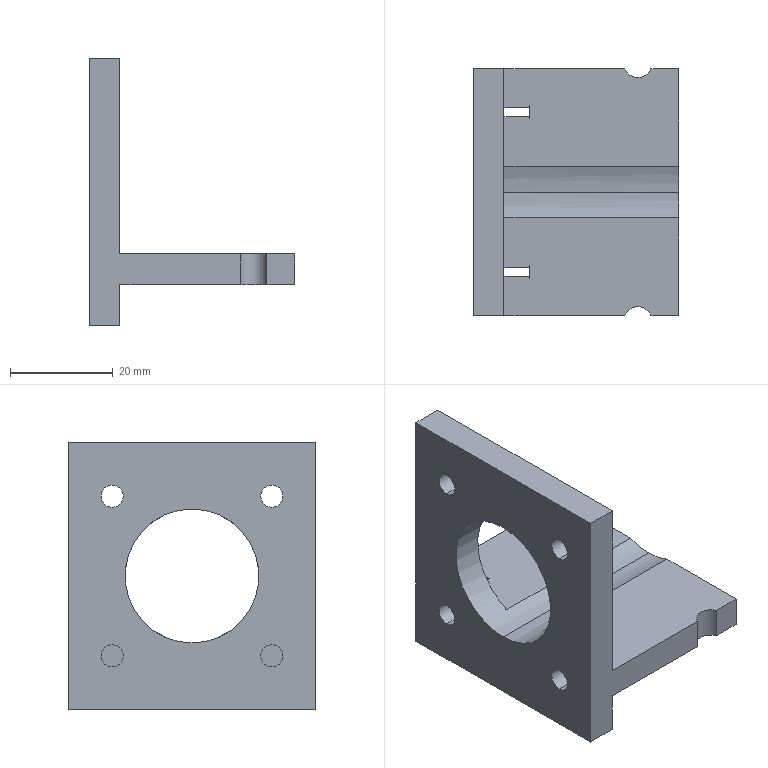Part | SolidWorks | features BaseBody 1 | 1 solid | 30 faces | box 40 x 48 x 52 mm | volume 20561 mm3 | cylinder 16 | plane 14 | commonest cylinder face diameters 4.3 x8 7.2 x4 5.5 x2 26 x2
STEP:
#1=CARTESIAN_POINT('',(0.,-15.5,31.35));
#2=VERTEX_POINT('',#1);
#3=CARTESIAN_POINT('',(0.,-15.5,35.65));
#4=VERTEX_POINT('',#3);
#5=CARTESIAN_POINT('',(0.,-15.5,33.5));
#6=DIRECTION('',(-1.,0.,0.));
#7=DIRECTION('',(0.,0.,-1.));
#8=AXIS2_PLACEMENT_3D('',#5,#6,#7);
#9=CIRCLE('',#8,2.15);
#10=EDGE_CURVE('',#2,#4,#9,.T.);
#11=ORIENTED_EDGE('',*,*,#10,.T.);
#12=CARTESIAN_POINT('',(6.,-15.5,35.65));
#13=VERTEX_POINT('',#12);
#14=CARTESIAN_POINT('',(-6.2,-15.5,35.65));
#15=DIRECTION('',(1.,0.,0.));
#16=VECTOR('',#15,1000.);
#17=LINE('',#14,#16);
#18=EDGE_CURVE('',#4,#13,#17,.T.);
#19=ORIENTED_EDGE('',*,*,#18,.T.);
#20=CARTESIAN_POINT('',(6.,-15.5,31.35));
#21=VERTEX_POINT('',#20);
#22=CARTESIAN_POINT('',(6.,-15.5,33.5));
#23=DIRECTION('',(-1.,0.,0.));
#24=DIRECTION('',(0.,0.,-1.));
#25=AXIS2_PLACEMENT_3D('',#22,#23,#24);
#26=CIRCLE('',#25,2.15);
#27=EDGE_CURVE('',#21,#13,#26,.T.);
#28=ORIENTED_EDGE('',*,*,#27,.F.);
#29=CARTESIAN_POINT('',(-6.2,-15.5,31.35));
#30=DIRECTION('',(1.,0.,0.));
#31=VECTOR('',#30,1000.);
#32=LINE('',#29,#31);
#33=EDGE_CURVE('',#2,#21,#32,.T.);
#34=ORIENTED_EDGE('',*,*,#33,.F.);
#35=EDGE_LOOP('',(#11,#19,#28,#34));
#36=FACE_OUTER_BOUND('',#35,.T.);
#37=CARTESIAN_POINT('',(-6.2,-15.5,33.5));
#38=DIRECTION('',(1.,0.,0.));
#39=DIRECTION('',(0.,0.,-1.));
#40=AXIS2_PLACEMENT_3D('',#37,#38,#39);
#41=CYLINDRICAL_SURFACE('',#40,2.15);
#42=ADVANCED_FACE('',(#36),#41,.F.);
#43=CARTESIAN_POINT('',(0.,0.,5.));
#44=VERTEX_POINT('',#43);
#45=CARTESIAN_POINT('',(0.,0.,31.));
#46=VERTEX_POINT('',#45);
#47=CARTESIAN_POINT('',(0.,0.,18.));
#48=DIRECTION('',(-1.,0.,0.));
#49=DIRECTION('',(0.,0.,-1.));
#50=AXIS2_PLACEMENT_3D('',#47,#48,#49);
#51=CIRCLE('',#50,13.);
#52=EDGE_CURVE('',#44,#46,#51,.T.);
#53=ORIENTED_EDGE('',*,*,#52,.T.);
#54=CARTESIAN_POINT('',(6.,0.,31.));
#55=VERTEX_POINT('',#54);
#56=CARTESIAN_POINT('',(-2.,0.,31.));
#57=DIRECTION('',(1.,0.,0.));
#58=VECTOR('',#57,1000.);
#59=LINE('',#56,#58);
#60=EDGE_CURVE('',#46,#55,#59,.T.);
#61=ORIENTED_EDGE('',*,*,#60,.T.);
#62=CARTESIAN_POINT('',(6.,-5.,6.));
#63=VERTEX_POINT('',#62);
#64=CARTESIAN_POINT('',(6.,0.,18.));
#65=DIRECTION('',(-1.,0.,0.));
#66=DIRECTION('',(0.,0.,-1.));
#67=AXIS2_PLACEMENT_3D('',#64,#65,#66);
#68=CIRCLE('',#67,13.);
#69=EDGE_CURVE('',#63,#55,#68,.T.);
#70=ORIENTED_EDGE('',*,*,#69,.F.);
#71=CARTESIAN_POINT('',(40.,-5.,6.));
#72=VERTEX_POINT('',#71);
#73=CARTESIAN_POINT('',(-2.,-5.,6.));
#74=DIRECTION('',(-1.,0.,0.));
#75=VECTOR('',#74,1000.);
#76=LINE('',#73,#75);
#77=EDGE_CURVE('',#72,#63,#76,.T.);
#78=ORIENTED_EDGE('',*,*,#77,.F.);
#79=CARTESIAN_POINT('',(40.,0.,5.));
#80=VERTEX_POINT('',#79);
#81=CARTESIAN_POINT('',(40.,0.,18.));
#82=DIRECTION('',(-1.,0.,0.));
#83=DIRECTION('',(0.,0.,-1.));
#84=AXIS2_PLACEMENT_3D('',#81,#82,#83);
#85=CIRCLE('',#84,13.);
#86=EDGE_CURVE('',#80,#72,#85,.T.);
#87=ORIENTED_EDGE('',*,*,#86,.F.);
#88=CARTESIAN_POINT('',(-2.,0.,5.));
#89=DIRECTION('',(1.,0.,0.));
#90=VECTOR('',#89,1000.);
#91=LINE('',#88,#90);
#92=EDGE_CURVE('',#44,#80,#91,.T.);
#93=ORIENTED_EDGE('',*,*,#92,.F.);
#94=EDGE_LOOP('',(#53,#61,#70,#78,#87,#93));
#95=FACE_OUTER_BOUND('',#94,.T.);
#96=CARTESIAN_POINT('',(-2.,0.,18.));
#97=DIRECTION('',(1.,0.,0.));
#98=DIRECTION('',(0.,0.,-1.));
#99=AXIS2_PLACEMENT_3D('',#96,#97,#98);
#100=CYLINDRICAL_SURFACE('',#99,13.);
#101=ADVANCED_FACE('',(#95),#100,.F.);
#102=CARTESIAN_POINT('',(0.,-15.5,0.35));
#103=VERTEX_POINT('',#102);
#104=CARTESIAN_POINT('',(0.,-15.5,4.65));
#105=VERTEX_POINT('',#104);
#106=CARTESIAN_POINT('',(0.,-15.5,2.5));
#107=DIRECTION('',(-1.,0.,0.));
#108=DIRECTION('',(0.,0.,-1.));
#109=AXIS2_PLACEMENT_3D('',#106,#107,#108);
#110=CIRCLE('',#109,2.15);
#111=EDGE_CURVE('',#103,#105,#110,.T.);
#112=ORIENTED_EDGE('',*,*,#111,.T.);
#113=CARTESIAN_POINT('',(6.,-15.5,4.65));
#114=VERTEX_POINT('',#113);
#115=CARTESIAN_POINT('',(-6.2,-15.5,4.65));
#116=DIRECTION('',(1.,0.,0.));
#117=VECTOR('',#116,1000.);
#118=LINE('',#115,#117);
#119=EDGE_CURVE('',#105,#114,#118,.T.);
#120=ORIENTED_EDGE('',*,*,#119,.T.);
#121=CARTESIAN_POINT('',(6.,-15.5,0.35));
#122=VERTEX_POINT('',#121);
#123=CARTESIAN_POINT('',(6.,-15.5,2.5));
#124=DIRECTION('',(-1.,0.,0.));
#125=DIRECTION('',(0.,0.,-1.));
#126=AXIS2_PLACEMENT_3D('',#123,#124,#125);
#127=CIRCLE('',#126,2.15);
#128=EDGE_CURVE('',#122,#114,#127,.T.);
#129=ORIENTED_EDGE('',*,*,#128,.F.);
#130=CARTESIAN_POINT('',(-6.2,-15.5,0.35));
#131=DIRECTION('',(1.,0.,0.));
#132=VECTOR('',#131,1000.);
#133=LINE('',#130,#132);
#134=EDGE_CURVE('',#103,#122,#133,.T.);
#135=ORIENTED_EDGE('',*,*,#134,.F.);
#136=EDGE_LOOP('',(#112,#120,#129,#135));
#137=FACE_OUTER_BOUND('',#136,.T.);
#138=CARTESIAN_POINT('',(-6.2,-15.5,2.5));
#139=DIRECTION('',(1.,0.,0.));
#140=DIRECTION('',(0.,0.,-1.));
#141=AXIS2_PLACEMENT_3D('',#138,#139,#140);
#142=CYLINDRICAL_SURFACE('',#141,2.15);
#143=ADVANCED_FACE('',(#137),#142,.F.);
#144=CARTESIAN_POINT('',(0.,15.5,31.35));
#145=VERTEX_POINT('',#144);
#146=CARTESIAN_POINT('',(0.,15.5,35.65));
#147=VERTEX_POINT('',#146);
#148=CARTESIAN_POINT('',(0.,15.5,33.5));
#149=DIRECTION('',(-1.,0.,0.));
#150=DIRECTION('',(0.,0.,-1.));
#151=AXIS2_PLACEMENT_3D('',#148,#149,#150);
#152=CIRCLE('',#151,2.15);
#153=EDGE_CURVE('',#145,#147,#152,.T.);
#154=ORIENTED_EDGE('',*,*,#153,.T.);
#155=CARTESIAN_POINT('',(6.,15.5,35.65));
#156=VERTEX_POINT('',#155);
#157=CARTESIAN_POINT('',(-6.2,15.5,35.65));
#158=DIRECTION('',(1.,0.,0.));
#159=VECTOR('',#158,1000.);
#160=LINE('',#157,#159);
#161=EDGE_CURVE('',#147,#156,#160,.T.);
#162=ORIENTED_EDGE('',*,*,#161,.T.);
#163=CARTESIAN_POINT('',(6.,15.5,31.35));
#164=VERTEX_POINT('',#163);
#165=CARTESIAN_POINT('',(6.,15.5,33.5));
#166=DIRECTION('',(-1.,0.,0.));
#167=DIRECTION('',(0.,0.,-1.));
#168=AXIS2_PLACEMENT_3D('',#165,#166,#167);
#169=CIRCLE('',#168,2.15);
#170=EDGE_CURVE('',#164,#156,#169,.T.);
#171=ORIENTED_EDGE('',*,*,#170,.F.);
#172=CARTESIAN_POINT('',(-6.2,15.5,31.35));
#173=DIRECTION('',(1.,0.,0.));
#174=VECTOR('',#173,1000.);
#175=LINE('',#172,#174);
#176=EDGE_CURVE('',#145,#164,#175,.T.);
#177=ORIENTED_EDGE('',*,*,#176,.F.);
#178=EDGE_LOOP('',(#154,#162,#171,#177));
#179=FACE_OUTER_BOUND('',#178,.T.);
#180=CARTESIAN_POINT('',(-6.2,15.5,33.5));
#181=DIRECTION('',(1.,0.,0.));
#182=DIRECTION('',(0.,0.,-1.));
#183=AXIS2_PLACEMENT_3D('',#180,#181,#182);
#184=CYLINDRICAL_SURFACE('',#183,2.15);
#185=ADVANCED_FACE('',(#179),#184,.F.);
#186=CARTESIAN_POINT('',(0.,15.5,0.35));
#187=VERTEX_POINT('',#186);
#188=CARTESIAN_POINT('',(0.,15.5,4.65));
#189=VERTEX_POINT('',#188);
#190=CARTESIAN_POINT('',(0.,15.5,2.5));
#191=DIRECTION('',(-1.,0.,0.));
#192=DIRECTION('',(0.,0.,-1.));
#193=AXIS2_PLACEMENT_3D('',#190,#191,#192);
#194=CIRCLE('',#193,2.15);
#195=EDGE_CURVE('',#187,#189,#194,.T.);
#196=ORIENTED_EDGE('',*,*,#195,.T.);
#197=CARTESIAN_POINT('',(6.,15.5,4.65));
#198=VERTEX_POINT('',#197);
#199=CARTESIAN_POINT('',(-6.2,15.5,4.65));
#200=DIRECTION('',(1.,0.,0.));
#201=VECTOR('',#200,1000.);
#202=LINE('',#199,#201);
#203=EDGE_CURVE('',#189,#198,#202,.T.);
#204=ORIENTED_EDGE('',*,*,#203,.T.);
#205=CARTESIAN_POINT('',(6.,15.5,0.35));
#206=VERTEX_POINT('',#205);
#207=CARTESIAN_POINT('',(6.,15.5,2.5));
#208=DIRECTION('',(-1.,0.,0.));
#209=DIRECTION('',(0.,0.,-1.));
#210=AXIS2_PLACEMENT_3D('',#207,#208,#209);
#211=CIRCLE('',#210,2.15);
#212=EDGE_CURVE('',#206,#198,#211,.T.);
#213=ORIENTED_EDGE('',*,*,#212,.F.);
#214=CARTESIAN_POINT('',(-6.2,15.5,0.35));
#215=DIRECTION('',(1.,0.,0.));
#216=VECTOR('',#215,1000.);
#217=LINE('',#214,#216);
#218=EDGE_CURVE('',#187,#206,#217,.T.);
#219=ORIENTED_EDGE('',*,*,#218,.F.);
#220=EDGE_LOOP('',(#196,#204,#213,#219));
#221=FACE_OUTER_BOUND('',#220,.T.);
#222=CARTESIAN_POINT('',(-6.2,15.5,2.5));
#223=DIRECTION('',(1.,0.,0.));
#224=DIRECTION('',(0.,0.,-1.));
#225=AXIS2_PLACEMENT_3D('',#222,#223,#224);
#226=CYLINDRICAL_SURFACE('',#225,2.15);
#227=ADVANCED_FACE('',(#221),#226,.F.);
#228=ORIENTED_EDGE('',*,*,#10,.F.);
#229=CARTESIAN_POINT('',(0.,-15.5,33.5));
#230=DIRECTION('',(-1.,0.,0.));
#231=DIRECTION('',(0.,0.,-1.));
#232=AXIS2_PLACEMENT_3D('',#229,#230,#231);
#233=CIRCLE('',#232,2.15);
#234=EDGE_CURVE('',#4,#2,#233,.T.);
#235=ORIENTED_EDGE('',*,*,#234,.F.);
#236=EDGE_LOOP('',(#228,#235));
#237=FACE_BOUND('',#236,.T.);
#238=ORIENTED_EDGE('',*,*,#52,.F.);
#239=CARTESIAN_POINT('',(0.,0.,18.));
#240=DIRECTION('',(-1.,0.,0.));
#241=DIRECTION('',(0.,0.,-1.));
#242=AXIS2_PLACEMENT_3D('',#239,#240,#241);
#243=CIRCLE('',#242,13.);
#244=EDGE_CURVE('',#46,#44,#243,.T.);
#245=ORIENTED_EDGE('',*,*,#244,.F.);
#246=EDGE_LOOP('',(#238,#245));
#247=FACE_BOUND('',#246,.T.);
#248=ORIENTED_EDGE('',*,*,#111,.F.);
#249=CARTESIAN_POINT('',(0.,-15.5,2.5));
#250=DIRECTION('',(-1.,0.,0.));
#251=DIRECTION('',(0.,0.,-1.));
#252=AXIS2_PLACEMENT_3D('',#249,#250,#251);
#253=CIRCLE('',#252,2.15);
#254=EDGE_CURVE('',#105,#103,#253,.T.);
#255=ORIENTED_EDGE('',*,*,#254,.F.);
#256=EDGE_LOOP('',(#248,#255));
#257=FACE_BOUND('',#256,.T.);
#258=ORIENTED_EDGE('',*,*,#153,.F.);
#259=CARTESIAN_POINT('',(0.,15.5,33.5));
#260=DIRECTION('',(-1.,0.,0.));
#261=DIRECTION('',(0.,0.,-1.));
#262=AXIS2_PLACEMENT_3D('',#259,#260,#261);
#263=CIRCLE('',#262,2.15);
#264=EDGE_CURVE('',#147,#145,#263,.T.);
#265=ORIENTED_EDGE('',*,*,#264,.F.);
#266=EDGE_LOOP('',(#258,#265));
#267=FACE_BOUND('',#266,.T.);
#268=ORIENTED_EDGE('',*,*,#195,.F.);
#269=CARTESIAN_POINT('',(0.,15.5,2.5));
#270=DIRECTION('',(-1.,0.,0.));
#271=DIRECTION('',(0.,0.,-1.));
#272=AXIS2_PLACEMENT_3D('',#269,#270,#271);
#273=CIRCLE('',#272,2.15);
#274=EDGE_CURVE('',#189,#187,#273,.T.);
#275=ORIENTED_EDGE('',*,*,#274,.F.);
#276=EDGE_LOOP('',(#268,#275));
#277=FACE_BOUND('',#276,.T.);
#278=CARTESIAN_POINT('',(0.,24.,-8.));
#279=VERTEX_POINT('',#278);
#280=CARTESIAN_POINT('',(0.,24.,44.));
#281=VERTEX_POINT('',#280);
#282=CARTESIAN_POINT('',(0.,24.,-8.));
#283=DIRECTION('',(0.,0.,1.));
#284=VECTOR('',#283,1000.);
#285=LINE('',#282,#284);
#286=EDGE_CURVE('',#279,#281,#285,.T.);
#287=ORIENTED_EDGE('',*,*,#286,.F.);
#288=CARTESIAN_POINT('',(0.,-24.,-8.));
#289=VERTEX_POINT('',#288);
#290=CARTESIAN_POINT('',(0.,-24.,-8.));
#291=DIRECTION('',(0.,1.,0.));
#292=VECTOR('',#291,1000.);
#293=LINE('',#290,#292);
#294=EDGE_CURVE('',#289,#279,#293,.T.);
#295=ORIENTED_EDGE('',*,*,#294,.F.);
#296=CARTESIAN_POINT('',(0.,-24.,44.));
#297=VERTEX_POINT('',#296);
#298=CARTESIAN_POINT('',(0.,-24.,-8.));
#299=DIRECTION('',(0.,0.,-1.));
#300=VECTOR('',#299,1000.);
#301=LINE('',#298,#300);
#302=EDGE_CURVE('',#297,#289,#301,.T.);
#303=ORIENTED_EDGE('',*,*,#302,.F.);
#304=CARTESIAN_POINT('',(0.,-24.,44.));
#305=DIRECTION('',(0.,-1.,0.));
#306=VECTOR('',#305,1000.);
#307=LINE('',#304,#306);
#308=EDGE_CURVE('',#281,#297,#307,.T.);
#309=ORIENTED_EDGE('',*,*,#308,.F.);
#310=EDGE_LOOP('',(#287,#295,#303,#309));
#311=FACE_OUTER_BOUND('',#310,.T.);
#312=CARTESIAN_POINT('',(0.,-24.,-8.));
#313=DIRECTION('',(1.,0.,0.));
#314=DIRECTION('',(0.,0.,-1.));
#315=AXIS2_PLACEMENT_3D('',#312,#313,#314);
#316=PLANE('',#315);
#317=ADVANCED_FACE('',(#237,#247,#257,#267,#277,#311),#316,.F.);
#318=ORIENTED_EDGE('',*,*,#18,.F.);
#319=ORIENTED_EDGE('',*,*,#234,.T.);
#320=ORIENTED_EDGE('',*,*,#33,.T.);
#321=CARTESIAN_POINT('',(6.,-15.5,33.5));
#322=DIRECTION('',(-1.,0.,0.));
#323=DIRECTION('',(0.,0.,-1.));
#324=AXIS2_PLACEMENT_3D('',#321,#322,#323);
#325=CIRCLE('',#324,2.15);
#326=EDGE_CURVE('',#13,#21,#325,.T.);
#327=ORIENTED_EDGE('',*,*,#326,.F.);
#328=EDGE_LOOP('',(#318,#319,#320,#327));
#329=FACE_OUTER_BOUND('',#328,.T.);
#330=CARTESIAN_POINT('',(-6.2,-15.5,33.5));
#331=DIRECTION('',(1.,0.,0.));
#332=DIRECTION('',(0.,0.,-1.));
#333=AXIS2_PLACEMENT_3D('',#330,#331,#332);
#334=CYLINDRICAL_SURFACE('',#333,2.15);
#335=ADVANCED_FACE('',(#329),#334,.F.);
#336=ORIENTED_EDGE('',*,*,#60,.F.);
#337=ORIENTED_EDGE('',*,*,#244,.T.);
#338=ORIENTED_EDGE('',*,*,#92,.T.);
#339=CARTESIAN_POINT('',(40.,5.,6.));
#340=VERTEX_POINT('',#339);
#341=CARTESIAN_POINT('',(40.,0.,18.));
#342=DIRECTION('',(-1.,0.,0.));
#343=DIRECTION('',(0.,0.,-1.));
#344=AXIS2_PLACEMENT_3D('',#341,#342,#343);
#345=CIRCLE('',#344,13.);
#346=EDGE_CURVE('',#340,#80,#345,.T.);
#347=ORIENTED_EDGE('',*,*,#346,.F.);
#348=CARTESIAN_POINT('',(6.,5.,6.));
#349=VERTEX_POINT('',#348);
#350=CARTESIAN_POINT('',(-2.,5.,6.));
#351=DIRECTION('',(1.,0.,0.));
#352=VECTOR('',#351,1000.);
#353=LINE('',#350,#352);
#354=EDGE_CURVE('',#349,#340,#353,.T.);
#355=ORIENTED_EDGE('',*,*,#354,.F.);
#356=CARTESIAN_POINT('',(6.,0.,18.));
#357=DIRECTION('',(-1.,0.,0.));
#358=DIRECTION('',(0.,0.,-1.));
#359=AXIS2_PLACEMENT_3D('',#356,#357,#358);
#360=CIRCLE('',#359,13.);
#361=EDGE_CURVE('',#55,#349,#360,.T.);
#362=ORIENTED_EDGE('',*,*,#361,.F.);
#363=EDGE_LOOP('',(#336,#337,#338,#347,#355,#362));
#364=FACE_OUTER_BOUND('',#363,.T.);
#365=CARTESIAN_POINT('',(-2.,0.,18.));
#366=DIRECTION('',(1.,0.,0.));
#367=DIRECTION('',(0.,0.,-1.));
#368=AXIS2_PLACEMENT_3D('',#365,#366,#367);
#369=CYLINDRICAL_SURFACE('',#368,13.);
#370=ADVANCED_FACE('',(#364),#369,.F.);
#371=ORIENTED_EDGE('',*,*,#119,.F.);
#372=ORIENTED_EDGE('',*,*,#254,.T.);
#373=ORIENTED_EDGE('',*,*,#134,.T.);
#374=CARTESIAN_POINT('',(6.,-15.5,2.5));
#375=DIRECTION('',(-1.,0.,0.));
#376=DIRECTION('',(0.,0.,-1.));
#377=AXIS2_PLACEMENT_3D('',#374,#375,#376);
#378=CIRCLE('',#377,2.15);
#379=EDGE_CURVE('',#114,#122,#378,.T.);
#380=ORIENTED_EDGE('',*,*,#379,.F.);
#381=EDGE_LOOP('',(#371,#372,#373,#380));
#382=FACE_OUTER_BOUND('',#381,.T.);
#383=CARTESIAN_POINT('',(-6.2,-15.5,2.5));
#384=DIRECTION('',(1.,0.,0.));
#385=DIRECTION('',(0.,0.,-1.));
#386=AXIS2_PLACEMENT_3D('',#383,#384,#385);
#387=CYLINDRICAL_SURFACE('',#386,2.15);
#388=ADVANCED_FACE('',(#382),#387,.F.);
#389=ORIENTED_EDGE('',*,*,#161,.F.);
#390=ORIENTED_EDGE('',*,*,#264,.T.);
#391=ORIENTED_EDGE('',*,*,#176,.T.);
#392=CARTESIAN_POINT('',(6.,15.5,33.5));
#393=DIRECTION('',(-1.,0.,0.));
#394=DIRECTION('',(0.,0.,-1.));
#395=AXIS2_PLACEMENT_3D('',#392,#393,#394);
#396=CIRCLE('',#395,2.15);
#397=EDGE_CURVE('',#156,#164,#396,.T.);
#398=ORIENTED_EDGE('',*,*,#397,.F.);
#399=EDGE_LOOP('',(#389,#390,#391,#398));
#400=FACE_OUTER_BOUND('',#399,.T.);
#401=CARTESIAN_POINT('',(-6.2,15.5,33.5));
#402=DIRECTION('',(1.,0.,0.));
#403=DIRECTION('',(0.,0.,-1.));
#404=AXIS2_PLACEMENT_3D('',#401,#402,#403);
#405=CYLINDRICAL_SURFACE('',#404,2.15);
#406=ADVANCED_FACE('',(#400),#405,.F.);
#407=ORIENTED_EDGE('',*,*,#203,.F.);
#408=ORIENTED_EDGE('',*,*,#274,.T.);
#409=ORIENTED_EDGE('',*,*,#218,.T.);
#410=CARTESIAN_POINT('',(6.,15.5,2.5));
#411=DIRECTION('',(-1.,0.,0.));
#412=DIRECTION('',(0.,0.,-1.));
#413=AXIS2_PLACEMENT_3D('',#410,#411,#412);
#414=CIRCLE('',#413,2.15);
#415=EDGE_CURVE('',#198,#206,#414,.T.);
#416=ORIENTED_EDGE('',*,*,#415,.F.);
#417=EDGE_LOOP('',(#407,#408,#409,#416));
#418=FACE_OUTER_BOUND('',#417,.T.);
#419=CARTESIAN_POINT('',(-6.2,15.5,2.5));
#420=DIRECTION('',(1.,0.,0.));
#421=DIRECTION('',(0.,0.,-1.));
#422=AXIS2_PLACEMENT_3D('',#419,#420,#421);
#423=CYLINDRICAL_SURFACE('',#422,2.15);
#424=ADVANCED_FACE('',(#418),#423,.F.);
#425=CARTESIAN_POINT('',(6.,-24.,44.));
#426=VERTEX_POINT('',#425);
#427=CARTESIAN_POINT('',(6.,24.,44.));
#428=VERTEX_POINT('',#427);
#429=CARTESIAN_POINT('',(6.,-24.,44.));
#430=DIRECTION('',(0.,1.,0.));
#431=VECTOR('',#430,1000.);
#432=LINE('',#429,#431);
#433=EDGE_CURVE('',#426,#428,#432,.T.);
#434=ORIENTED_EDGE('',*,*,#433,.T.);
#435=CARTESIAN_POINT('',(0.,24.,44.));
#436=DIRECTION('',(-1.,0.,0.));
#437=VECTOR('',#436,1000.);
#438=LINE('',#435,#437);
#439=EDGE_CURVE('',#428,#281,#438,.T.);
#440=ORIENTED_EDGE('',*,*,#439,.T.);
#441=ORIENTED_EDGE('',*,*,#308,.T.);
#442=CARTESIAN_POINT('',(0.,-24.,44.));
#443=DIRECTION('',(1.,0.,0.));
#444=VECTOR('',#443,1000.);
#445=LINE('',#442,#444);
#446=EDGE_CURVE('',#297,#426,#445,.T.);
#447=ORIENTED_EDGE('',*,*,#446,.T.);
#448=EDGE_LOOP('',(#434,#440,#441,#447));
#449=FACE_OUTER_BOUND('',#448,.T.);
#450=CARTESIAN_POINT('',(0.,-24.,44.));
#451=DIRECTION('',(0.,0.,1.));
#452=DIRECTION('',(1.,0.,0.));
#453=AXIS2_PLACEMENT_3D('',#450,#451,#452);
#454=PLANE('',#453);
#455=ADVANCED_FACE('',(#449),#454,.T.);
#456=CARTESIAN_POINT('',(29.438,24.,6.));
#457=VERTEX_POINT('',#456);
#458=CARTESIAN_POINT('',(29.438,24.,0.));
#459=VERTEX_POINT('',#458);
#460=CARTESIAN_POINT('',(29.438,24.,-8.));
#461=DIRECTION('',(0.,0.,-1.));
#462=VECTOR('',#461,1000.);
#463=LINE('',#460,#462);
#464=EDGE_CURVE('',#457,#459,#463,.T.);
#465=ORIENTED_EDGE('',*,*,#464,.T.);
#466=CARTESIAN_POINT('',(6.,24.,0.));
#467=VERTEX_POINT('',#466);
#468=CARTESIAN_POINT('',(0.,24.,0.));
#469=DIRECTION('',(-1.,0.,0.));
#470=VECTOR('',#469,1000.);
#471=LINE('',#468,#470);
#472=EDGE_CURVE('',#459,#467,#471,.T.);
#473=ORIENTED_EDGE('',*,*,#472,.T.);
#474=CARTESIAN_POINT('',(6.,24.,-8.));
#475=VERTEX_POINT('',#474);
#476=CARTESIAN_POINT('',(6.,24.,-8.));
#477=DIRECTION('',(0.,0.,-1.));
#478=VECTOR('',#477,1000.);
#479=LINE('',#476,#478);
#480=EDGE_CURVE('',#467,#475,#479,.T.);
#481=ORIENTED_EDGE('',*,*,#480,.T.);
#482=CARTESIAN_POINT('',(0.,24.,-8.));
#483=DIRECTION('',(-1.,0.,0.));
#484=VECTOR('',#483,1000.);
#485=LINE('',#482,#484);
#486=EDGE_CURVE('',#475,#279,#485,.T.);
#487=ORIENTED_EDGE('',*,*,#486,.T.);
#488=ORIENTED_EDGE('',*,*,#286,.T.);
#489=ORIENTED_EDGE('',*,*,#439,.F.);
#490=CARTESIAN_POINT('',(6.,24.,6.));
#491=VERTEX_POINT('',#490);
#492=CARTESIAN_POINT('',(6.,24.,-8.));
#493=DIRECTION('',(0.,0.,-1.));
#494=VECTOR('',#493,1000.);
#495=LINE('',#492,#494);
#496=EDGE_CURVE('',#428,#491,#495,.T.);
#497=ORIENTED_EDGE('',*,*,#496,.T.);
#498=CARTESIAN_POINT('',(0.,24.,6.));
#499=DIRECTION('',(1.,0.,0.));
#500=VECTOR('',#499,1000.);
#501=LINE('',#498,#500);
#502=EDGE_CURVE('',#491,#457,#501,.T.);
#503=ORIENTED_EDGE('',*,*,#502,.T.);
#504=EDGE_LOOP('',(#465,#473,#481,#487,#488,#489,#497,#503));
#505=FACE_OUTER_BOUND('',#504,.T.);
#506=CARTESIAN_POINT('',(0.,24.,-8.));
#507=DIRECTION('',(0.,1.,0.));
#508=DIRECTION('',(0.,0.,1.));
#509=AXIS2_PLACEMENT_3D('',#506,#507,#508);
#510=PLANE('',#509);
#511=ADVANCED_FACE('',(#505),#510,.T.);
#512=CARTESIAN_POINT('',(6.,-24.,-8.));
#513=VERTEX_POINT('',#512);
#514=CARTESIAN_POINT('',(6.,-24.,-8.));
#515=DIRECTION('',(0.,1.,0.));
#516=VECTOR('',#515,1000.);
#517=LINE('',#514,#516);
#518=EDGE_CURVE('',#513,#475,#517,.T.);
#519=ORIENTED_EDGE('',*,*,#518,.F.);
#520=CARTESIAN_POINT('',(0.,-24.,-8.));
#521=DIRECTION('',(1.,0.,0.));
#522=VECTOR('',#521,1000.);
#523=LINE('',#520,#522);
#524=EDGE_CURVE('',#289,#513,#523,.T.);
#525=ORIENTED_EDGE('',*,*,#524,.F.);
#526=ORIENTED_EDGE('',*,*,#294,.T.);
#527=ORIENTED_EDGE('',*,*,#486,.F.);
#528=EDGE_LOOP('',(#519,#525,#526,#527));
#529=FACE_OUTER_BOUND('',#528,.T.);
#530=CARTESIAN_POINT('',(0.,-24.,-8.));
#531=DIRECTION('',(0.,0.,1.));
#532=DIRECTION('',(1.,0.,0.));
#533=AXIS2_PLACEMENT_3D('',#530,#531,#532);
#534=PLANE('',#533);
#535=ADVANCED_FACE('',(#529),#534,.F.);
#536=CARTESIAN_POINT('',(29.438,-24.,6.));
#537=VERTEX_POINT('',#536);
#538=CARTESIAN_POINT('',(29.438,-24.,0.));
#539=VERTEX_POINT('',#538);
#540=CARTESIAN_POINT('',(29.438,-24.,-8.));
#541=DIRECTION('',(0.,0.,-1.));
#542=VECTOR('',#541,1000.);
#543=LINE('',#540,#542);
#544=EDGE_CURVE('',#537,#539,#543,.T.);
#545=ORIENTED_EDGE('',*,*,#544,.F.);
#546=CARTESIAN_POINT('',(6.,-24.,6.));
#547=VERTEX_POINT('',#546);
#548=CARTESIAN_POINT('',(0.,-24.,6.));
#549=DIRECTION('',(1.,0.,0.));
#550=VECTOR('',#549,1000.);
#551=LINE('',#548,#550);
#552=EDGE_CURVE('',#547,#537,#551,.T.);
#553=ORIENTED_EDGE('',*,*,#552,.F.);
#554=CARTESIAN_POINT('',(6.,-24.,-8.));
#555=DIRECTION('',(0.,0.,-1.));
#556=VECTOR('',#555,1000.);
#557=LINE('',#554,#556);
#558=EDGE_CURVE('',#426,#547,#557,.T.);
#559=ORIENTED_EDGE('',*,*,#558,.F.);
#560=ORIENTED_EDGE('',*,*,#446,.F.);
#561=ORIENTED_EDGE('',*,*,#302,.T.);
#562=ORIENTED_EDGE('',*,*,#524,.T.);
#563=CARTESIAN_POINT('',(6.,-24.,0.));
#564=VERTEX_POINT('',#563);
#565=CARTESIAN_POINT('',(6.,-24.,-8.));
#566=DIRECTION('',(0.,0.,-1.));
#567=VECTOR('',#566,1000.);
#568=LINE('',#565,#567);
#569=EDGE_CURVE('',#564,#513,#568,.T.);
#570=ORIENTED_EDGE('',*,*,#569,.F.);
#571=CARTESIAN_POINT('',(0.,-24.,0.));
#572=DIRECTION('',(-1.,0.,0.));
#573=VECTOR('',#572,1000.);
#574=LINE('',#571,#573);
#575=EDGE_CURVE('',#539,#564,#574,.T.);
#576=ORIENTED_EDGE('',*,*,#575,.F.);
#577=EDGE_LOOP('',(#545,#553,#559,#560,#561,#562,#570,#576));
#578=FACE_OUTER_BOUND('',#577,.T.);
#579=CARTESIAN_POINT('',(0.,-24.,-8.));
#580=DIRECTION('',(0.,1.,0.));
#581=DIRECTION('',(0.,0.,1.));
#582=AXIS2_PLACEMENT_3D('',#579,#580,#581);
#583=PLANE('',#582);
#584=ADVANCED_FACE('',(#578),#583,.F.);
#585=ORIENTED_EDGE('',*,*,#27,.T.);
#586=ORIENTED_EDGE('',*,*,#326,.T.);
#587=EDGE_LOOP('',(#585,#586));
#588=FACE_BOUND('',#587,.T.);
#589=ORIENTED_EDGE('',*,*,#128,.T.);
#590=ORIENTED_EDGE('',*,*,#379,.T.);
#591=EDGE_LOOP('',(#589,#590));
#592=FACE_BOUND('',#591,.T.);
#593=CARTESIAN_POINT('',(6.,-14.657,6.));
#594=VERTEX_POINT('',#593);
#595=CARTESIAN_POINT('',(6.,-24.,6.));
#596=DIRECTION('',(0.,1.,0.));
#597=VECTOR('',#596,1000.);
#598=LINE('',#595,#597);
#599=EDGE_CURVE('',#594,#63,#598,.T.);
#600=ORIENTED_EDGE('',*,*,#599,.T.);
#601=ORIENTED_EDGE('',*,*,#69,.T.);
#602=ORIENTED_EDGE('',*,*,#361,.T.);
#603=CARTESIAN_POINT('',(6.,14.657,6.));
#604=VERTEX_POINT('',#603);
#605=CARTESIAN_POINT('',(6.,-24.,6.));
#606=DIRECTION('',(0.,1.,0.));
#607=VECTOR('',#606,1000.);
#608=LINE('',#605,#607);
#609=EDGE_CURVE('',#349,#604,#608,.T.);
#610=ORIENTED_EDGE('',*,*,#609,.T.);
#611=CARTESIAN_POINT('',(6.,12.91,0.));
#612=VERTEX_POINT('',#611);
#613=CARTESIAN_POINT('',(6.,15.5,2.5));
#614=DIRECTION('',(1.,0.,0.));
#615=DIRECTION('',(0.,0.,-1.));
#616=AXIS2_PLACEMENT_3D('',#613,#614,#615);
#617=CIRCLE('',#616,3.6);
#618=EDGE_CURVE('',#604,#612,#617,.T.);
#619=ORIENTED_EDGE('',*,*,#618,.T.);
#620=CARTESIAN_POINT('',(6.,-12.91,0.));
#621=VERTEX_POINT('',#620);
#622=CARTESIAN_POINT('',(6.,-24.,0.));
#623=DIRECTION('',(0.,-1.,0.));
#624=VECTOR('',#623,1000.);
#625=LINE('',#622,#624);
#626=EDGE_CURVE('',#612,#621,#625,.T.);
#627=ORIENTED_EDGE('',*,*,#626,.T.);
#628=CARTESIAN_POINT('',(6.,-15.5,2.5));
#629=DIRECTION('',(1.,0.,0.));
#630=DIRECTION('',(0.,0.,-1.));
#631=AXIS2_PLACEMENT_3D('',#628,#629,#630);
#632=CIRCLE('',#631,3.6);
#633=EDGE_CURVE('',#621,#594,#632,.T.);
#634=ORIENTED_EDGE('',*,*,#633,.T.);
#635=EDGE_LOOP('',(#600,#601,#602,#610,#619,#627,#634));
#636=FACE_BOUND('',#635,.T.);
#637=ORIENTED_EDGE('',*,*,#170,.T.);
#638=ORIENTED_EDGE('',*,*,#397,.T.);
#639=EDGE_LOOP('',(#637,#638));
#640=FACE_BOUND('',#639,.T.);
#641=ORIENTED_EDGE('',*,*,#212,.T.);
#642=ORIENTED_EDGE('',*,*,#415,.T.);
#643=EDGE_LOOP('',(#641,#642));
#644=FACE_BOUND('',#643,.T.);
#645=CARTESIAN_POINT('',(6.,-16.343,6.));
#646=VERTEX_POINT('',#645);
#647=CARTESIAN_POINT('',(6.,-18.09,0.));
#648=VERTEX_POINT('',#647);
#649=CARTESIAN_POINT('',(6.,-15.5,2.5));
#650=DIRECTION('',(1.,0.,0.));
#651=DIRECTION('',(0.,0.,-1.));
#652=AXIS2_PLACEMENT_3D('',#649,#650,#651);
#653=CIRCLE('',#652,3.6);
#654=EDGE_CURVE('',#646,#648,#653,.T.);
#655=ORIENTED_EDGE('',*,*,#654,.T.);
#656=CARTESIAN_POINT('',(6.,-24.,0.));
#657=DIRECTION('',(0.,-1.,0.));
#658=VECTOR('',#657,1000.);
#659=LINE('',#656,#658);
#660=EDGE_CURVE('',#648,#564,#659,.T.);
#661=ORIENTED_EDGE('',*,*,#660,.T.);
#662=ORIENTED_EDGE('',*,*,#569,.T.);
#663=ORIENTED_EDGE('',*,*,#518,.T.);
#664=ORIENTED_EDGE('',*,*,#480,.F.);
#665=CARTESIAN_POINT('',(6.,18.09,0.));
#666=VERTEX_POINT('',#665);
#667=CARTESIAN_POINT('',(6.,-24.,0.));
#668=DIRECTION('',(0.,-1.,0.));
#669=VECTOR('',#668,1000.);
#670=LINE('',#667,#669);
#671=EDGE_CURVE('',#467,#666,#670,.T.);
#672=ORIENTED_EDGE('',*,*,#671,.T.);
#673=CARTESIAN_POINT('',(6.,16.343,6.));
#674=VERTEX_POINT('',#673);
#675=CARTESIAN_POINT('',(6.,15.5,2.5));
#676=DIRECTION('',(1.,0.,0.));
#677=DIRECTION('',(0.,0.,-1.));
#678=AXIS2_PLACEMENT_3D('',#675,#676,#677);
#679=CIRCLE('',#678,3.6);
#680=EDGE_CURVE('',#666,#674,#679,.T.);
#681=ORIENTED_EDGE('',*,*,#680,.T.);
#682=CARTESIAN_POINT('',(6.,-24.,6.));
#683=DIRECTION('',(0.,1.,0.));
#684=VECTOR('',#683,1000.);
#685=LINE('',#682,#684);
#686=EDGE_CURVE('',#674,#491,#685,.T.);
#687=ORIENTED_EDGE('',*,*,#686,.T.);
#688=ORIENTED_EDGE('',*,*,#496,.F.);
#689=ORIENTED_EDGE('',*,*,#433,.F.);
#690=ORIENTED_EDGE('',*,*,#558,.T.);
#691=CARTESIAN_POINT('',(6.,-24.,6.));
#692=DIRECTION('',(0.,1.,0.));
#693=VECTOR('',#692,1000.);
#694=LINE('',#691,#693);
#695=EDGE_CURVE('',#547,#646,#694,.T.);
#696=ORIENTED_EDGE('',*,*,#695,.T.);
#697=EDGE_LOOP('',(#655,#661,#662,#663,#664,#672,#681,#687,#688,#689,#690,#696));
#698=FACE_OUTER_BOUND('',#697,.T.);
#699=CARTESIAN_POINT('',(6.,-24.,-8.));
#700=DIRECTION('',(1.,0.,0.));
#701=DIRECTION('',(0.,0.,-1.));
#702=AXIS2_PLACEMENT_3D('',#699,#700,#701);
#703=PLANE('',#702);
#704=ADVANCED_FACE('',(#588,#592,#636,#640,#644,#698),#703,.T.);
#705=CARTESIAN_POINT('',(34.562,-24.,6.));
#706=VERTEX_POINT('',#705);
#707=CARTESIAN_POINT('',(40.,-24.,6.));
#708=VERTEX_POINT('',#707);
#709=CARTESIAN_POINT('',(0.,-24.,6.));
#710=DIRECTION('',(1.,0.,0.));
#711=VECTOR('',#710,1000.);
#712=LINE('',#709,#711);
#713=EDGE_CURVE('',#706,#708,#712,.T.);
#714=ORIENTED_EDGE('',*,*,#713,.T.);
#715=CARTESIAN_POINT('',(40.,-24.,6.));
#716=DIRECTION('',(0.,1.,0.));
#717=VECTOR('',#716,1000.);
#718=LINE('',#715,#717);
#719=EDGE_CURVE('',#708,#72,#718,.T.);
#720=ORIENTED_EDGE('',*,*,#719,.T.);
#721=ORIENTED_EDGE('',*,*,#77,.T.);
#722=ORIENTED_EDGE('',*,*,#599,.F.);
#723=CARTESIAN_POINT('',(11.,-14.657,6.));
#724=VERTEX_POINT('',#723);
#725=CARTESIAN_POINT('',(0.,-14.657,6.));
#726=DIRECTION('',(1.,0.,0.));
#727=VECTOR('',#726,1000.);
#728=LINE('',#725,#727);
#729=EDGE_CURVE('',#594,#724,#728,.T.);
#730=ORIENTED_EDGE('',*,*,#729,.T.);
#731=CARTESIAN_POINT('',(11.,-16.343,6.));
#732=VERTEX_POINT('',#731);
#733=CARTESIAN_POINT('',(11.,-15.5,6.));
#734=DIRECTION('',(0.,-1.,0.));
#735=VECTOR('',#734,1000.);
#736=LINE('',#733,#735);
#737=EDGE_CURVE('',#724,#732,#736,.T.);
#738=ORIENTED_EDGE('',*,*,#737,.T.);
#739=CARTESIAN_POINT('',(0.,-16.343,6.));
#740=DIRECTION('',(-1.,0.,0.));
#741=VECTOR('',#740,1000.);
#742=LINE('',#739,#741);
#743=EDGE_CURVE('',#732,#646,#742,.T.);
#744=ORIENTED_EDGE('',*,*,#743,.T.);
#745=ORIENTED_EDGE('',*,*,#695,.F.);
#746=ORIENTED_EDGE('',*,*,#552,.T.);
#747=CARTESIAN_POINT('',(32.,-25.,6.));
#748=DIRECTION('',(0.,0.,-1.));
#749=DIRECTION('',(1.,0.,0.));
#750=AXIS2_PLACEMENT_3D('',#747,#748,#749);
#751=CIRCLE('',#750,2.75);
#752=EDGE_CURVE('',#537,#706,#751,.T.);
#753=ORIENTED_EDGE('',*,*,#752,.T.);
#754=EDGE_LOOP('',(#714,#720,#721,#722,#730,#738,#744,#745,#746,#753));
#755=FACE_OUTER_BOUND('',#754,.T.);
#756=CARTESIAN_POINT('',(0.,-24.,6.));
#757=DIRECTION('',(0.,0.,1.));
#758=DIRECTION('',(1.,0.,0.));
#759=AXIS2_PLACEMENT_3D('',#756,#757,#758);
#760=PLANE('',#759);
#761=ADVANCED_FACE('',(#755),#760,.T.);
#762=CARTESIAN_POINT('',(40.,24.,6.));
#763=VERTEX_POINT('',#762);
#764=CARTESIAN_POINT('',(40.,-24.,6.));
#765=DIRECTION('',(0.,-1.,0.));
#766=VECTOR('',#765,1000.);
#767=LINE('',#764,#766);
#768=EDGE_CURVE('',#763,#340,#767,.T.);
#769=ORIENTED_EDGE('',*,*,#768,.T.);
#770=ORIENTED_EDGE('',*,*,#346,.T.);
#771=ORIENTED_EDGE('',*,*,#86,.T.);
#772=ORIENTED_EDGE('',*,*,#719,.F.);
#773=CARTESIAN_POINT('',(40.,-24.,0.));
#774=VERTEX_POINT('',#773);
#775=CARTESIAN_POINT('',(40.,-24.,0.));
#776=DIRECTION('',(0.,0.,-1.));
#777=VECTOR('',#776,1000.);
#778=LINE('',#775,#777);
#779=EDGE_CURVE('',#708,#774,#778,.T.);
#780=ORIENTED_EDGE('',*,*,#779,.T.);
#781=CARTESIAN_POINT('',(40.,24.,0.));
#782=VERTEX_POINT('',#781);
#783=CARTESIAN_POINT('',(40.,-24.,0.));
#784=DIRECTION('',(0.,1.,0.));
#785=VECTOR('',#784,1000.);
#786=LINE('',#783,#785);
#787=EDGE_CURVE('',#774,#782,#786,.T.);
#788=ORIENTED_EDGE('',*,*,#787,.T.);
#789=CARTESIAN_POINT('',(40.,24.,0.));
#790=DIRECTION('',(0.,0.,1.));
#791=VECTOR('',#790,1000.);
#792=LINE('',#789,#791);
#793=EDGE_CURVE('',#782,#763,#792,.T.);
#794=ORIENTED_EDGE('',*,*,#793,.T.);
#795=EDGE_LOOP('',(#769,#770,#771,#772,#780,#788,#794));
#796=FACE_OUTER_BOUND('',#795,.T.);
#797=CARTESIAN_POINT('',(40.,-24.,0.));
#798=DIRECTION('',(1.,0.,0.));
#799=DIRECTION('',(0.,0.,-1.));
#800=AXIS2_PLACEMENT_3D('',#797,#798,#799);
#801=PLANE('',#800);
#802=ADVANCED_FACE('',(#796),#801,.T.);
#803=CARTESIAN_POINT('',(34.562,24.,6.));
#804=VERTEX_POINT('',#803);
#805=CARTESIAN_POINT('',(0.,24.,6.));
#806=DIRECTION('',(-1.,0.,0.));
#807=VECTOR('',#806,1000.);
#808=LINE('',#805,#807);
#809=EDGE_CURVE('',#763,#804,#808,.T.);
#810=ORIENTED_EDGE('',*,*,#809,.T.);
#811=CARTESIAN_POINT('',(32.,25.,6.));
#812=DIRECTION('',(0.,0.,-1.));
#813=DIRECTION('',(1.,0.,0.));
#814=AXIS2_PLACEMENT_3D('',#811,#812,#813);
#815=CIRCLE('',#814,2.75);
#816=EDGE_CURVE('',#804,#457,#815,.T.);
#817=ORIENTED_EDGE('',*,*,#816,.T.);
#818=ORIENTED_EDGE('',*,*,#502,.F.);
#819=ORIENTED_EDGE('',*,*,#686,.F.);
#820=CARTESIAN_POINT('',(11.,16.343,6.));
#821=VERTEX_POINT('',#820);
#822=CARTESIAN_POINT('',(0.,16.343,6.));
#823=DIRECTION('',(1.,0.,0.));
#824=VECTOR('',#823,1000.);
#825=LINE('',#822,#824);
#826=EDGE_CURVE('',#674,#821,#825,.T.);
#827=ORIENTED_EDGE('',*,*,#826,.T.);
#828=CARTESIAN_POINT('',(11.,14.657,6.));
#829=VERTEX_POINT('',#828);
#830=CARTESIAN_POINT('',(11.,15.5,6.));
#831=DIRECTION('',(0.,-1.,0.));
#832=VECTOR('',#831,1000.);
#833=LINE('',#830,#832);
#834=EDGE_CURVE('',#821,#829,#833,.T.);
#835=ORIENTED_EDGE('',*,*,#834,.T.);
#836=CARTESIAN_POINT('',(0.,14.657,6.));
#837=DIRECTION('',(-1.,0.,0.));
#838=VECTOR('',#837,1000.);
#839=LINE('',#836,#838);
#840=EDGE_CURVE('',#829,#604,#839,.T.);
#841=ORIENTED_EDGE('',*,*,#840,.T.);
#842=ORIENTED_EDGE('',*,*,#609,.F.);
#843=ORIENTED_EDGE('',*,*,#354,.T.);
#844=ORIENTED_EDGE('',*,*,#768,.F.);
#845=EDGE_LOOP('',(#810,#817,#818,#819,#827,#835,#841,#842,#843,#844));
#846=FACE_OUTER_BOUND('',#845,.T.);
#847=CARTESIAN_POINT('',(0.,-24.,6.));
#848=DIRECTION('',(0.,0.,1.));
#849=DIRECTION('',(1.,0.,0.));
#850=AXIS2_PLACEMENT_3D('',#847,#848,#849);
#851=PLANE('',#850);
#852=ADVANCED_FACE('',(#846),#851,.T.);
#853=CARTESIAN_POINT('',(34.562,24.,0.));
#854=VERTEX_POINT('',#853);
#855=CARTESIAN_POINT('',(0.,24.,0.));
#856=DIRECTION('',(-1.,0.,0.));
#857=VECTOR('',#856,1000.);
#858=LINE('',#855,#857);
#859=EDGE_CURVE('',#782,#854,#858,.T.);
#860=ORIENTED_EDGE('',*,*,#859,.F.);
#861=ORIENTED_EDGE('',*,*,#787,.F.);
#862=CARTESIAN_POINT('',(34.562,-24.,0.));
#863=VERTEX_POINT('',#862);
#864=CARTESIAN_POINT('',(0.,-24.,0.));
#865=DIRECTION('',(1.,0.,0.));
#866=VECTOR('',#865,1000.);
#867=LINE('',#864,#866);
#868=EDGE_CURVE('',#863,#774,#867,.T.);
#869=ORIENTED_EDGE('',*,*,#868,.F.);
#870=CARTESIAN_POINT('',(32.,-25.,0.));
#871=DIRECTION('',(0.,0.,-1.));
#872=DIRECTION('',(1.,0.,0.));
#873=AXIS2_PLACEMENT_3D('',#870,#871,#872);
#874=CIRCLE('',#873,2.75);
#875=EDGE_CURVE('',#539,#863,#874,.T.);
#876=ORIENTED_EDGE('',*,*,#875,.F.);
#877=ORIENTED_EDGE('',*,*,#575,.T.);
#878=ORIENTED_EDGE('',*,*,#660,.F.);
#879=CARTESIAN_POINT('',(11.,-18.09,0.));
#880=VERTEX_POINT('',#879);
#881=CARTESIAN_POINT('',(0.,-18.09,0.));
#882=DIRECTION('',(-1.,0.,0.));
#883=VECTOR('',#882,1000.);
#884=LINE('',#881,#883);
#885=EDGE_CURVE('',#880,#648,#884,.T.);
#886=ORIENTED_EDGE('',*,*,#885,.F.);
#887=CARTESIAN_POINT('',(11.,-12.91,0.));
#888=VERTEX_POINT('',#887);
#889=CARTESIAN_POINT('',(11.,-24.,0.));
#890=DIRECTION('',(0.,-1.,0.));
#891=VECTOR('',#890,1000.);
#892=LINE('',#889,#891);
#893=EDGE_CURVE('',#888,#880,#892,.T.);
#894=ORIENTED_EDGE('',*,*,#893,.F.);
#895=CARTESIAN_POINT('',(0.,-12.91,0.));
#896=DIRECTION('',(1.,0.,0.));
#897=VECTOR('',#896,1000.);
#898=LINE('',#895,#897);
#899=EDGE_CURVE('',#621,#888,#898,.T.);
#900=ORIENTED_EDGE('',*,*,#899,.F.);
#901=ORIENTED_EDGE('',*,*,#626,.F.);
#902=CARTESIAN_POINT('',(11.,12.91,0.));
#903=VERTEX_POINT('',#902);
#904=CARTESIAN_POINT('',(0.,12.91,0.));
#905=DIRECTION('',(-1.,0.,0.));
#906=VECTOR('',#905,1000.);
#907=LINE('',#904,#906);
#908=EDGE_CURVE('',#903,#612,#907,.T.);
#909=ORIENTED_EDGE('',*,*,#908,.F.);
#910=CARTESIAN_POINT('',(11.,18.09,0.));
#911=VERTEX_POINT('',#910);
#912=CARTESIAN_POINT('',(11.,-24.,0.));
#913=DIRECTION('',(0.,-1.,0.));
#914=VECTOR('',#913,1000.);
#915=LINE('',#912,#914);
#916=EDGE_CURVE('',#911,#903,#915,.T.);
#917=ORIENTED_EDGE('',*,*,#916,.F.);
#918=CARTESIAN_POINT('',(0.,18.09,0.));
#919=DIRECTION('',(1.,0.,0.));
#920=VECTOR('',#919,1000.);
#921=LINE('',#918,#920);
#922=EDGE_CURVE('',#666,#911,#921,.T.);
#923=ORIENTED_EDGE('',*,*,#922,.F.);
#924=ORIENTED_EDGE('',*,*,#671,.F.);
#925=ORIENTED_EDGE('',*,*,#472,.F.);
#926=CARTESIAN_POINT('',(32.,25.,0.));
#927=DIRECTION('',(0.,0.,-1.));
#928=DIRECTION('',(1.,0.,0.));
#929=AXIS2_PLACEMENT_3D('',#926,#927,#928);
#930=CIRCLE('',#929,2.75);
#931=EDGE_CURVE('',#854,#459,#930,.T.);
#932=ORIENTED_EDGE('',*,*,#931,.F.);
#933=EDGE_LOOP('',(#860,#861,#869,#876,#877,#878,#886,#894,#900,#901,#909,#917,#923,#924,#925,#932));
#934=FACE_OUTER_BOUND('',#933,.T.);
#935=CARTESIAN_POINT('',(0.,-24.,0.));
#936=DIRECTION('',(0.,0.,1.));
#937=DIRECTION('',(1.,0.,0.));
#938=AXIS2_PLACEMENT_3D('',#935,#936,#937);
#939=PLANE('',#938);
#940=ADVANCED_FACE('',(#934),#939,.F.);
#941=ORIENTED_EDGE('',*,*,#816,.F.);
#942=CARTESIAN_POINT('',(34.562,24.,-1.));
#943=DIRECTION('',(0.,0.,1.));
#944=VECTOR('',#943,1000.);
#945=LINE('',#942,#944);
#946=EDGE_CURVE('',#854,#804,#945,.T.);
#947=ORIENTED_EDGE('',*,*,#946,.F.);
#948=ORIENTED_EDGE('',*,*,#931,.T.);
#949=ORIENTED_EDGE('',*,*,#464,.F.);
#950=EDGE_LOOP('',(#941,#947,#948,#949));
#951=FACE_OUTER_BOUND('',#950,.T.);
#952=CARTESIAN_POINT('',(32.,25.,-1.));
#953=DIRECTION('',(0.,0.,1.));
#954=DIRECTION('',(1.,0.,0.));
#955=AXIS2_PLACEMENT_3D('',#952,#953,#954);
#956=CYLINDRICAL_SURFACE('',#955,2.75);
#957=ADVANCED_FACE('',(#951),#956,.F.);
#958=ORIENTED_EDGE('',*,*,#544,.T.);
#959=ORIENTED_EDGE('',*,*,#875,.T.);
#960=CARTESIAN_POINT('',(34.562,-24.,-1.));
#961=DIRECTION('',(0.,0.,-1.));
#962=VECTOR('',#961,1000.);
#963=LINE('',#960,#962);
#964=EDGE_CURVE('',#706,#863,#963,.T.);
#965=ORIENTED_EDGE('',*,*,#964,.F.);
#966=ORIENTED_EDGE('',*,*,#752,.F.);
#967=EDGE_LOOP('',(#958,#959,#965,#966));
#968=FACE_OUTER_BOUND('',#967,.T.);
#969=CARTESIAN_POINT('',(32.,-25.,-1.));
#970=DIRECTION('',(0.,0.,1.));
#971=DIRECTION('',(1.,0.,0.));
#972=AXIS2_PLACEMENT_3D('',#969,#970,#971);
#973=CYLINDRICAL_SURFACE('',#972,2.75);
#974=ADVANCED_FACE('',(#968),#973,.F.);
#975=ORIENTED_EDGE('',*,*,#633,.F.);
#976=ORIENTED_EDGE('',*,*,#899,.T.);
#977=CARTESIAN_POINT('',(11.,-15.5,2.5));
#978=DIRECTION('',(-1.,0.,0.));
#979=DIRECTION('',(0.,0.,-1.));
#980=AXIS2_PLACEMENT_3D('',#977,#978,#979);
#981=CIRCLE('',#980,3.6);
#982=EDGE_CURVE('',#724,#888,#981,.T.);
#983=ORIENTED_EDGE('',*,*,#982,.F.);
#984=ORIENTED_EDGE('',*,*,#729,.F.);
#985=EDGE_LOOP('',(#975,#976,#983,#984));
#986=FACE_OUTER_BOUND('',#985,.T.);
#987=CARTESIAN_POINT('',(6.,-15.5,2.5));
#988=DIRECTION('',(1.,0.,0.));
#989=DIRECTION('',(0.,0.,-1.));
#990=AXIS2_PLACEMENT_3D('',#987,#988,#989);
#991=CYLINDRICAL_SURFACE('',#990,3.6);
#992=ADVANCED_FACE('',(#986),#991,.F.);
#993=ORIENTED_EDGE('',*,*,#840,.F.);
#994=CARTESIAN_POINT('',(11.,15.5,2.5));
#995=DIRECTION('',(-1.,0.,0.));
#996=DIRECTION('',(0.,0.,-1.));
#997=AXIS2_PLACEMENT_3D('',#994,#995,#996);
#998=CIRCLE('',#997,3.6);
#999=EDGE_CURVE('',#903,#829,#998,.T.);
#1000=ORIENTED_EDGE('',*,*,#999,.F.);
#1001=ORIENTED_EDGE('',*,*,#908,.T.);
#1002=ORIENTED_EDGE('',*,*,#618,.F.);
#1003=EDGE_LOOP('',(#993,#1000,#1001,#1002));
#1004=FACE_OUTER_BOUND('',#1003,.T.);
#1005=CARTESIAN_POINT('',(6.,15.5,2.5));
#1006=DIRECTION('',(1.,0.,0.));
#1007=DIRECTION('',(0.,0.,-1.));
#1008=AXIS2_PLACEMENT_3D('',#1005,#1006,#1007);
#1009=CYLINDRICAL_SURFACE('',#1008,3.6);
#1010=ADVANCED_FACE('',(#1004),#1009,.F.);
#1011=ORIENTED_EDGE('',*,*,#743,.F.);
#1012=CARTESIAN_POINT('',(11.,-15.5,2.5));
#1013=DIRECTION('',(-1.,0.,0.));
#1014=DIRECTION('',(0.,0.,-1.));
#1015=AXIS2_PLACEMENT_3D('',#1012,#1013,#1014);
#1016=CIRCLE('',#1015,3.6);
#1017=EDGE_CURVE('',#880,#732,#1016,.T.);
#1018=ORIENTED_EDGE('',*,*,#1017,.F.);
#1019=ORIENTED_EDGE('',*,*,#885,.T.);
#1020=ORIENTED_EDGE('',*,*,#654,.F.);
#1021=EDGE_LOOP('',(#1011,#1018,#1019,#1020));
#1022=FACE_OUTER_BOUND('',#1021,.T.);
#1023=CARTESIAN_POINT('',(6.,-15.5,2.5));
#1024=DIRECTION('',(1.,0.,0.));
#1025=DIRECTION('',(0.,0.,-1.));
#1026=AXIS2_PLACEMENT_3D('',#1023,#1024,#1025);
#1027=CYLINDRICAL_SURFACE('',#1026,3.6);
#1028=ADVANCED_FACE('',(#1022),#1027,.F.);
#1029=ORIENTED_EDGE('',*,*,#680,.F.);
#1030=ORIENTED_EDGE('',*,*,#922,.T.);
#1031=CARTESIAN_POINT('',(11.,15.5,2.5));
#1032=DIRECTION('',(-1.,0.,0.));
#1033=DIRECTION('',(0.,0.,-1.));
#1034=AXIS2_PLACEMENT_3D('',#1031,#1032,#1033);
#1035=CIRCLE('',#1034,3.6);
#1036=EDGE_CURVE('',#821,#911,#1035,.T.);
#1037=ORIENTED_EDGE('',*,*,#1036,.F.);
#1038=ORIENTED_EDGE('',*,*,#826,.F.);
#1039=EDGE_LOOP('',(#1029,#1030,#1037,#1038));
#1040=FACE_OUTER_BOUND('',#1039,.T.);
#1041=CARTESIAN_POINT('',(6.,15.5,2.5));
#1042=DIRECTION('',(1.,0.,0.));
#1043=DIRECTION('',(0.,0.,-1.));
#1044=AXIS2_PLACEMENT_3D('',#1041,#1042,#1043);
#1045=CYLINDRICAL_SURFACE('',#1044,3.6);
#1046=ADVANCED_FACE('',(#1040),#1045,.F.);
#1047=ORIENTED_EDGE('',*,*,#713,.F.);
#1048=ORIENTED_EDGE('',*,*,#964,.T.);
#1049=ORIENTED_EDGE('',*,*,#868,.T.);
#1050=ORIENTED_EDGE('',*,*,#779,.F.);
#1051=EDGE_LOOP('',(#1047,#1048,#1049,#1050));
#1052=FACE_OUTER_BOUND('',#1051,.T.);
#1053=CARTESIAN_POINT('',(0.,-24.,-8.));
#1054=DIRECTION('',(0.,1.,0.));
#1055=DIRECTION('',(0.,0.,1.));
#1056=AXIS2_PLACEMENT_3D('',#1053,#1054,#1055);
#1057=PLANE('',#1056);
#1058=ADVANCED_FACE('',(#1052),#1057,.F.);
#1059=ORIENTED_EDGE('',*,*,#809,.F.);
#1060=ORIENTED_EDGE('',*,*,#793,.F.);
#1061=ORIENTED_EDGE('',*,*,#859,.T.);
#1062=ORIENTED_EDGE('',*,*,#946,.T.);
#1063=EDGE_LOOP('',(#1059,#1060,#1061,#1062));
#1064=FACE_OUTER_BOUND('',#1063,.T.);
#1065=CARTESIAN_POINT('',(0.,24.,-8.));
#1066=DIRECTION('',(0.,1.,0.));
#1067=DIRECTION('',(0.,0.,1.));
#1068=AXIS2_PLACEMENT_3D('',#1065,#1066,#1067);
#1069=PLANE('',#1068);
#1070=ADVANCED_FACE('',(#1064),#1069,.T.);
#1071=ORIENTED_EDGE('',*,*,#737,.F.);
#1072=ORIENTED_EDGE('',*,*,#982,.T.);
#1073=ORIENTED_EDGE('',*,*,#893,.T.);
#1074=ORIENTED_EDGE('',*,*,#1017,.T.);
#1075=EDGE_LOOP('',(#1071,#1072,#1073,#1074));
#1076=FACE_OUTER_BOUND('',#1075,.T.);
#1077=CARTESIAN_POINT('',(11.,-15.5,2.5));
#1078=DIRECTION('',(1.,0.,0.));
#1079=DIRECTION('',(0.,0.,-1.));
#1080=AXIS2_PLACEMENT_3D('',#1077,#1078,#1079);
#1081=PLANE('',#1080);
#1082=ADVANCED_FACE('',(#1076),#1081,.F.);
#1083=ORIENTED_EDGE('',*,*,#834,.F.);
#1084=ORIENTED_EDGE('',*,*,#1036,.T.);
#1085=ORIENTED_EDGE('',*,*,#916,.T.);
#1086=ORIENTED_EDGE('',*,*,#999,.T.);
#1087=EDGE_LOOP('',(#1083,#1084,#1085,#1086));
#1088=FACE_OUTER_BOUND('',#1087,.T.);
#1089=CARTESIAN_POINT('',(11.,15.5,2.5));
#1090=DIRECTION('',(1.,0.,0.));
#1091=DIRECTION('',(0.,0.,-1.));
#1092=AXIS2_PLACEMENT_3D('',#1089,#1090,#1091);
#1093=PLANE('',#1092);
#1094=ADVANCED_FACE('',(#1088),#1093,.F.);
#1095=CLOSED_SHELL('',(#42,#101,#143,#185,#227,#317,#335,#370,#388,#406,#424,#455,#511,#535,#584,#704,#761,#802,#852,#940,#957,#974,#992,#1010,#1028,#1046,#1058,#1070,#1082,#1094));
#1096=MANIFOLD_SOLID_BREP('',#1095);
#1097=CARTESIAN_POINT('',(0.,0.,0.));
#1098=DIRECTION('',(0.,0.,1.));
#1099=DIRECTION('',(1.,0.,0.));
#1100=AXIS2_PLACEMENT_3D('',#1097,#1098,#1099);
#1101=(LENGTH_UNIT()NAMED_UNIT(*)SI_UNIT(.MILLI.,.METRE.));
#1102=UNCERTAINTY_MEASURE_WITH_UNIT(LENGTH_MEASURE(0.00001),#1101,'','');
#1103=(NAMED_UNIT(*)PLANE_ANGLE_UNIT()SI_UNIT($,.RADIAN.));
#1104=(NAMED_UNIT(*)SI_UNIT($,.STERADIAN.)SOLID_ANGLE_UNIT());
#1105=(GEOMETRIC_REPRESENTATION_CONTEXT(3)GLOBAL_UNCERTAINTY_ASSIGNED_CONTEXT((#1102))GLOBAL_UNIT_ASSIGNED_CONTEXT((#1101,#1103,#1104))REPRESENTATION_CONTEXT('',''));
#1106=ADVANCED_BREP_SHAPE_REPRESENTATION('',(#1096,#1100),#1105);